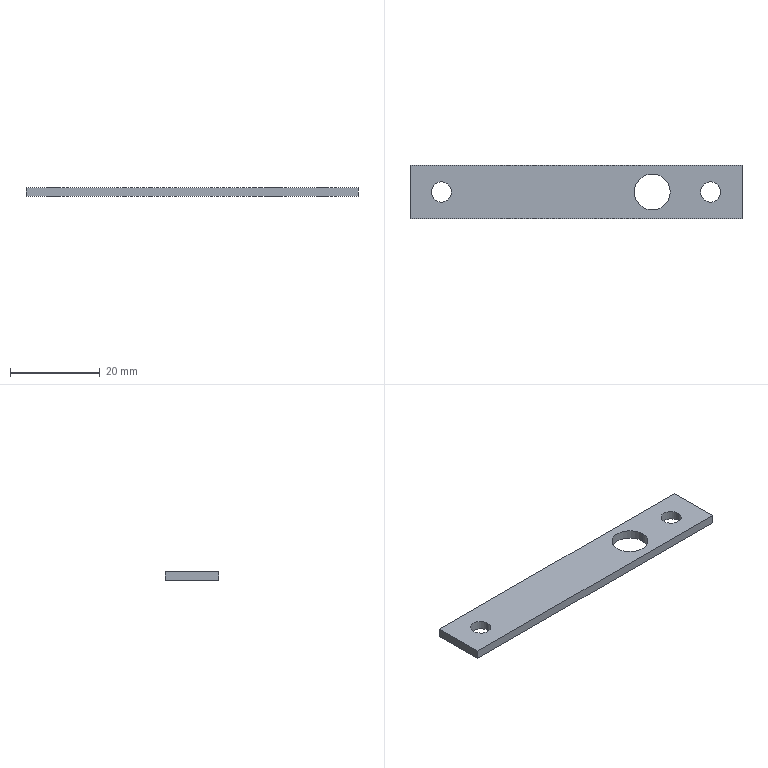Part | Creo | features DATUM PLANE 3, COORDINATE SYSTEM 1, CURVE 1, PROTRUSION 1 | 1 solid | 12 faces | box 74 x 12 x 2 mm | volume 1612 mm3 | plane 6 | cylinder 6 | commonest cylinder face diameters 4.5 x4 8 x2
STEP:
#1=CARTESIAN_POINT('',(0.,0.,0.));
#2=DIRECTION('',(0.,0.,1.));
#3=DIRECTION('',(1.,0.,0.));
#4=AXIS2_PLACEMENT_3D('',#1,#2,#3);
#5=CARTESIAN_POINT('',(-54.,6.,0.));
#6=VERTEX_POINT('',#5);
#7=CARTESIAN_POINT('',(-54.,-6.,0.));
#8=VERTEX_POINT('',#7);
#9=CARTESIAN_POINT('',(-54.,6.,0.));
#10=DIRECTION('',(0.,-1.,0.));
#11=VECTOR('',#10,12.);
#12=LINE('',#9,#11);
#13=EDGE_CURVE('',#6,#8,#12,.T.);
#14=ORIENTED_EDGE('',*,*,#13,.T.);
#15=CARTESIAN_POINT('',(20.,-6.,0.));
#16=VERTEX_POINT('',#15);
#17=CARTESIAN_POINT('',(-54.,-6.,0.));
#18=DIRECTION('',(1.,0.,0.));
#19=VECTOR('',#18,74.);
#20=LINE('',#17,#19);
#21=EDGE_CURVE('',#8,#16,#20,.T.);
#22=ORIENTED_EDGE('',*,*,#21,.T.);
#23=CARTESIAN_POINT('',(20.,6.,0.));
#24=VERTEX_POINT('',#23);
#25=CARTESIAN_POINT('',(20.,-6.,0.));
#26=DIRECTION('',(0.,1.,0.));
#27=VECTOR('',#26,12.);
#28=LINE('',#25,#27);
#29=EDGE_CURVE('',#16,#24,#28,.T.);
#30=ORIENTED_EDGE('',*,*,#29,.T.);
#31=CARTESIAN_POINT('',(20.,6.,0.));
#32=DIRECTION('',(-1.,0.,0.));
#33=VECTOR('',#32,74.);
#34=LINE('',#31,#33);
#35=EDGE_CURVE('',#24,#6,#34,.T.);
#36=ORIENTED_EDGE('',*,*,#35,.T.);
#37=EDGE_LOOP('',(#14,#22,#30,#36));
#38=FACE_OUTER_BOUND('',#37,.F.);
#39=CARTESIAN_POINT('',(15.25,0.,0.));
#40=VERTEX_POINT('',#39);
#41=CARTESIAN_POINT('',(10.75,0.,0.));
#42=VERTEX_POINT('',#41);
#43=CARTESIAN_POINT('',(13.,0.,0.));
#44=DIRECTION('',(0.,0.,-1.));
#45=DIRECTION('',(1.,0.,0.));
#46=AXIS2_PLACEMENT_3D('',#43,#44,#45);
#47=CIRCLE('',#46,2.25);
#48=EDGE_CURVE('',#40,#42,#47,.T.);
#49=ORIENTED_EDGE('',*,*,#48,.T.);
#50=CARTESIAN_POINT('',(13.,0.,0.));
#51=DIRECTION('',(0.,0.,-1.));
#52=DIRECTION('',(-1.,0.,0.));
#53=AXIS2_PLACEMENT_3D('',#50,#51,#52);
#54=CIRCLE('',#53,2.25);
#55=EDGE_CURVE('',#42,#40,#54,.T.);
#56=ORIENTED_EDGE('',*,*,#55,.T.);
#57=EDGE_LOOP('',(#49,#56));
#58=FACE_BOUND('',#57,.F.);
#59=CARTESIAN_POINT('',(-44.75,0.,0.));
#60=VERTEX_POINT('',#59);
#61=CARTESIAN_POINT('',(-49.25,0.,0.));
#62=VERTEX_POINT('',#61);
#63=CARTESIAN_POINT('',(-47.,0.,0.));
#64=DIRECTION('',(0.,0.,-1.));
#65=DIRECTION('',(1.,0.,0.));
#66=AXIS2_PLACEMENT_3D('',#63,#64,#65);
#67=CIRCLE('',#66,2.25);
#68=EDGE_CURVE('',#60,#62,#67,.T.);
#69=ORIENTED_EDGE('',*,*,#68,.T.);
#70=CARTESIAN_POINT('',(-47.,0.,0.));
#71=DIRECTION('',(0.,0.,-1.));
#72=DIRECTION('',(-1.,0.,0.));
#73=AXIS2_PLACEMENT_3D('',#70,#71,#72);
#74=CIRCLE('',#73,2.25);
#75=EDGE_CURVE('',#62,#60,#74,.T.);
#76=ORIENTED_EDGE('',*,*,#75,.T.);
#77=EDGE_LOOP('',(#69,#76));
#78=FACE_BOUND('',#77,.F.);
#79=CARTESIAN_POINT('',(4.,0.,0.));
#80=VERTEX_POINT('',#79);
#81=CARTESIAN_POINT('',(-4.,0.,0.));
#82=VERTEX_POINT('',#81);
#83=CARTESIAN_POINT('',(0.,0.,0.));
#84=DIRECTION('',(0.,0.,-1.));
#85=DIRECTION('',(1.,0.,0.));
#86=AXIS2_PLACEMENT_3D('',#83,#84,#85);
#87=CIRCLE('',#86,4.);
#88=EDGE_CURVE('',#80,#82,#87,.T.);
#89=ORIENTED_EDGE('',*,*,#88,.T.);
#90=CARTESIAN_POINT('',(0.,0.,0.));
#91=DIRECTION('',(0.,0.,-1.));
#92=DIRECTION('',(-1.,0.,0.));
#93=AXIS2_PLACEMENT_3D('',#90,#91,#92);
#94=CIRCLE('',#93,4.);
#95=EDGE_CURVE('',#82,#80,#94,.T.);
#96=ORIENTED_EDGE('',*,*,#95,.T.);
#97=EDGE_LOOP('',(#89,#96));
#98=FACE_BOUND('',#97,.F.);
#99=CARTESIAN_POINT('',(0.,0.,0.));
#100=DIRECTION('',(0.,0.,1.));
#101=DIRECTION('',(1.,0.,0.));
#102=AXIS2_PLACEMENT_3D('',#99,#100,#101);
#103=PLANE('',#102);
#104=ADVANCED_FACE('',(#38,#58,#78,#98),#103,.F.);
#105=ORIENTED_EDGE('',*,*,#88,.F.);
#106=CARTESIAN_POINT('',(4.,0.,2.));
#107=VERTEX_POINT('',#106);
#108=CARTESIAN_POINT('',(4.,0.,0.));
#109=DIRECTION('',(0.,0.,1.));
#110=VECTOR('',#109,2.);
#111=LINE('',#108,#110);
#112=EDGE_CURVE('',#80,#107,#111,.T.);
#113=ORIENTED_EDGE('',*,*,#112,.T.);
#114=CARTESIAN_POINT('',(-4.,0.,2.));
#115=VERTEX_POINT('',#114);
#116=CARTESIAN_POINT('',(0.,0.,2.));
#117=DIRECTION('',(0.,0.,-1.));
#118=DIRECTION('',(1.,0.,0.));
#119=AXIS2_PLACEMENT_3D('',#116,#117,#118);
#120=CIRCLE('',#119,4.);
#121=EDGE_CURVE('',#107,#115,#120,.T.);
#122=ORIENTED_EDGE('',*,*,#121,.T.);
#123=CARTESIAN_POINT('',(-4.,0.,0.));
#124=DIRECTION('',(0.,0.,1.));
#125=VECTOR('',#124,2.);
#126=LINE('',#123,#125);
#127=EDGE_CURVE('',#82,#115,#126,.T.);
#128=ORIENTED_EDGE('',*,*,#127,.F.);
#129=EDGE_LOOP('',(#105,#113,#122,#128));
#130=FACE_OUTER_BOUND('',#129,.F.);
#131=CARTESIAN_POINT('',(0.,0.,0.));
#132=DIRECTION('',(0.,0.,1.));
#133=DIRECTION('',(1.,0.,0.));
#134=AXIS2_PLACEMENT_3D('',#131,#132,#133);
#135=CYLINDRICAL_SURFACE('',#134,4.);
#136=ADVANCED_FACE('',(#130),#135,.F.);
#137=ORIENTED_EDGE('',*,*,#95,.F.);
#138=ORIENTED_EDGE('',*,*,#127,.T.);
#139=CARTESIAN_POINT('',(0.,0.,2.));
#140=DIRECTION('',(0.,0.,-1.));
#141=DIRECTION('',(-1.,0.,0.));
#142=AXIS2_PLACEMENT_3D('',#139,#140,#141);
#143=CIRCLE('',#142,4.);
#144=EDGE_CURVE('',#115,#107,#143,.T.);
#145=ORIENTED_EDGE('',*,*,#144,.T.);
#146=ORIENTED_EDGE('',*,*,#112,.F.);
#147=EDGE_LOOP('',(#137,#138,#145,#146));
#148=FACE_OUTER_BOUND('',#147,.F.);
#149=CARTESIAN_POINT('',(0.,0.,0.));
#150=DIRECTION('',(0.,0.,1.));
#151=DIRECTION('',(1.,0.,0.));
#152=AXIS2_PLACEMENT_3D('',#149,#150,#151);
#153=CYLINDRICAL_SURFACE('',#152,4.);
#154=ADVANCED_FACE('',(#148),#153,.F.);
#155=CARTESIAN_POINT('',(-54.,6.,2.));
#156=VERTEX_POINT('',#155);
#157=CARTESIAN_POINT('',(-54.,-6.,2.));
#158=VERTEX_POINT('',#157);
#159=CARTESIAN_POINT('',(-54.,6.,2.));
#160=DIRECTION('',(0.,-1.,0.));
#161=VECTOR('',#160,12.);
#162=LINE('',#159,#161);
#163=EDGE_CURVE('',#156,#158,#162,.T.);
#164=ORIENTED_EDGE('',*,*,#163,.F.);
#165=CARTESIAN_POINT('',(20.,6.,2.));
#166=VERTEX_POINT('',#165);
#167=CARTESIAN_POINT('',(20.,6.,2.));
#168=DIRECTION('',(-1.,0.,0.));
#169=VECTOR('',#168,74.);
#170=LINE('',#167,#169);
#171=EDGE_CURVE('',#166,#156,#170,.T.);
#172=ORIENTED_EDGE('',*,*,#171,.F.);
#173=CARTESIAN_POINT('',(20.,-6.,2.));
#174=VERTEX_POINT('',#173);
#175=CARTESIAN_POINT('',(20.,-6.,2.));
#176=DIRECTION('',(0.,1.,0.));
#177=VECTOR('',#176,12.);
#178=LINE('',#175,#177);
#179=EDGE_CURVE('',#174,#166,#178,.T.);
#180=ORIENTED_EDGE('',*,*,#179,.F.);
#181=CARTESIAN_POINT('',(-54.,-6.,2.));
#182=DIRECTION('',(1.,0.,0.));
#183=VECTOR('',#182,74.);
#184=LINE('',#181,#183);
#185=EDGE_CURVE('',#158,#174,#184,.T.);
#186=ORIENTED_EDGE('',*,*,#185,.F.);
#187=EDGE_LOOP('',(#164,#172,#180,#186));
#188=FACE_OUTER_BOUND('',#187,.F.);
#189=CARTESIAN_POINT('',(15.25,0.,2.));
#190=VERTEX_POINT('',#189);
#191=CARTESIAN_POINT('',(10.75,0.,2.));
#192=VERTEX_POINT('',#191);
#193=CARTESIAN_POINT('',(13.,0.,2.));
#194=DIRECTION('',(0.,0.,-1.));
#195=DIRECTION('',(1.,0.,0.));
#196=AXIS2_PLACEMENT_3D('',#193,#194,#195);
#197=CIRCLE('',#196,2.25);
#198=EDGE_CURVE('',#190,#192,#197,.T.);
#199=ORIENTED_EDGE('',*,*,#198,.F.);
#200=CARTESIAN_POINT('',(13.,0.,2.));
#201=DIRECTION('',(0.,0.,-1.));
#202=DIRECTION('',(-1.,0.,0.));
#203=AXIS2_PLACEMENT_3D('',#200,#201,#202);
#204=CIRCLE('',#203,2.25);
#205=EDGE_CURVE('',#192,#190,#204,.T.);
#206=ORIENTED_EDGE('',*,*,#205,.F.);
#207=EDGE_LOOP('',(#199,#206));
#208=FACE_BOUND('',#207,.F.);
#209=CARTESIAN_POINT('',(-44.75,0.,2.));
#210=VERTEX_POINT('',#209);
#211=CARTESIAN_POINT('',(-49.25,0.,2.));
#212=VERTEX_POINT('',#211);
#213=CARTESIAN_POINT('',(-47.,0.,2.));
#214=DIRECTION('',(0.,0.,-1.));
#215=DIRECTION('',(1.,0.,0.));
#216=AXIS2_PLACEMENT_3D('',#213,#214,#215);
#217=CIRCLE('',#216,2.25);
#218=EDGE_CURVE('',#210,#212,#217,.T.);
#219=ORIENTED_EDGE('',*,*,#218,.F.);
#220=CARTESIAN_POINT('',(-47.,0.,2.));
#221=DIRECTION('',(0.,0.,-1.));
#222=DIRECTION('',(-1.,0.,0.));
#223=AXIS2_PLACEMENT_3D('',#220,#221,#222);
#224=CIRCLE('',#223,2.25);
#225=EDGE_CURVE('',#212,#210,#224,.T.);
#226=ORIENTED_EDGE('',*,*,#225,.F.);
#227=EDGE_LOOP('',(#219,#226));
#228=FACE_BOUND('',#227,.F.);
#229=ORIENTED_EDGE('',*,*,#121,.F.);
#230=ORIENTED_EDGE('',*,*,#144,.F.);
#231=EDGE_LOOP('',(#229,#230));
#232=FACE_BOUND('',#231,.F.);
#233=CARTESIAN_POINT('',(0.,0.,2.));
#234=DIRECTION('',(0.,0.,1.));
#235=DIRECTION('',(1.,0.,0.));
#236=AXIS2_PLACEMENT_3D('',#233,#234,#235);
#237=PLANE('',#236);
#238=ADVANCED_FACE('',(#188,#208,#228,#232),#237,.T.);
#239=ORIENTED_EDGE('',*,*,#48,.F.);
#240=CARTESIAN_POINT('',(15.25,0.,0.));
#241=DIRECTION('',(0.,0.,1.));
#242=VECTOR('',#241,2.);
#243=LINE('',#240,#242);
#244=EDGE_CURVE('',#40,#190,#243,.T.);
#245=ORIENTED_EDGE('',*,*,#244,.T.);
#246=ORIENTED_EDGE('',*,*,#198,.T.);
#247=CARTESIAN_POINT('',(10.75,0.,0.));
#248=DIRECTION('',(0.,0.,1.));
#249=VECTOR('',#248,2.);
#250=LINE('',#247,#249);
#251=EDGE_CURVE('',#42,#192,#250,.T.);
#252=ORIENTED_EDGE('',*,*,#251,.F.);
#253=EDGE_LOOP('',(#239,#245,#246,#252));
#254=FACE_OUTER_BOUND('',#253,.F.);
#255=CARTESIAN_POINT('',(13.,0.,0.));
#256=DIRECTION('',(0.,0.,1.));
#257=DIRECTION('',(1.,0.,0.));
#258=AXIS2_PLACEMENT_3D('',#255,#256,#257);
#259=CYLINDRICAL_SURFACE('',#258,2.25);
#260=ADVANCED_FACE('',(#254),#259,.F.);
#261=ORIENTED_EDGE('',*,*,#55,.F.);
#262=ORIENTED_EDGE('',*,*,#251,.T.);
#263=ORIENTED_EDGE('',*,*,#205,.T.);
#264=ORIENTED_EDGE('',*,*,#244,.F.);
#265=EDGE_LOOP('',(#261,#262,#263,#264));
#266=FACE_OUTER_BOUND('',#265,.F.);
#267=CARTESIAN_POINT('',(13.,0.,0.));
#268=DIRECTION('',(0.,0.,1.));
#269=DIRECTION('',(1.,0.,0.));
#270=AXIS2_PLACEMENT_3D('',#267,#268,#269);
#271=CYLINDRICAL_SURFACE('',#270,2.25);
#272=ADVANCED_FACE('',(#266),#271,.F.);
#273=ORIENTED_EDGE('',*,*,#68,.F.);
#274=CARTESIAN_POINT('',(-44.75,0.,0.));
#275=DIRECTION('',(0.,0.,1.));
#276=VECTOR('',#275,2.);
#277=LINE('',#274,#276);
#278=EDGE_CURVE('',#60,#210,#277,.T.);
#279=ORIENTED_EDGE('',*,*,#278,.T.);
#280=ORIENTED_EDGE('',*,*,#218,.T.);
#281=CARTESIAN_POINT('',(-49.25,0.,0.));
#282=DIRECTION('',(0.,0.,1.));
#283=VECTOR('',#282,2.);
#284=LINE('',#281,#283);
#285=EDGE_CURVE('',#62,#212,#284,.T.);
#286=ORIENTED_EDGE('',*,*,#285,.F.);
#287=EDGE_LOOP('',(#273,#279,#280,#286));
#288=FACE_OUTER_BOUND('',#287,.F.);
#289=CARTESIAN_POINT('',(-47.,0.,0.));
#290=DIRECTION('',(0.,0.,1.));
#291=DIRECTION('',(1.,0.,0.));
#292=AXIS2_PLACEMENT_3D('',#289,#290,#291);
#293=CYLINDRICAL_SURFACE('',#292,2.25);
#294=ADVANCED_FACE('',(#288),#293,.F.);
#295=ORIENTED_EDGE('',*,*,#75,.F.);
#296=ORIENTED_EDGE('',*,*,#285,.T.);
#297=ORIENTED_EDGE('',*,*,#225,.T.);
#298=ORIENTED_EDGE('',*,*,#278,.F.);
#299=EDGE_LOOP('',(#295,#296,#297,#298));
#300=FACE_OUTER_BOUND('',#299,.F.);
#301=CARTESIAN_POINT('',(-47.,0.,0.));
#302=DIRECTION('',(0.,0.,1.));
#303=DIRECTION('',(1.,0.,0.));
#304=AXIS2_PLACEMENT_3D('',#301,#302,#303);
#305=CYLINDRICAL_SURFACE('',#304,2.25);
#306=ADVANCED_FACE('',(#300),#305,.F.);
#307=ORIENTED_EDGE('',*,*,#13,.F.);
#308=CARTESIAN_POINT('',(-54.,6.,0.));
#309=DIRECTION('',(0.,0.,1.));
#310=VECTOR('',#309,2.);
#311=LINE('',#308,#310);
#312=EDGE_CURVE('',#6,#156,#311,.T.);
#313=ORIENTED_EDGE('',*,*,#312,.T.);
#314=ORIENTED_EDGE('',*,*,#163,.T.);
#315=CARTESIAN_POINT('',(-54.,-6.,0.));
#316=DIRECTION('',(0.,0.,1.));
#317=VECTOR('',#316,2.);
#318=LINE('',#315,#317);
#319=EDGE_CURVE('',#8,#158,#318,.T.);
#320=ORIENTED_EDGE('',*,*,#319,.F.);
#321=EDGE_LOOP('',(#307,#313,#314,#320));
#322=FACE_OUTER_BOUND('',#321,.F.);
#323=CARTESIAN_POINT('',(-54.,6.,0.));
#324=DIRECTION('',(-1.,0.,0.));
#325=DIRECTION('',(0.,-1.,0.));
#326=AXIS2_PLACEMENT_3D('',#323,#324,#325);
#327=PLANE('',#326);
#328=ADVANCED_FACE('',(#322),#327,.T.);
#329=ORIENTED_EDGE('',*,*,#35,.F.);
#330=CARTESIAN_POINT('',(20.,6.,0.));
#331=DIRECTION('',(0.,0.,1.));
#332=VECTOR('',#331,2.);
#333=LINE('',#330,#332);
#334=EDGE_CURVE('',#24,#166,#333,.T.);
#335=ORIENTED_EDGE('',*,*,#334,.T.);
#336=ORIENTED_EDGE('',*,*,#171,.T.);
#337=ORIENTED_EDGE('',*,*,#312,.F.);
#338=EDGE_LOOP('',(#329,#335,#336,#337));
#339=FACE_OUTER_BOUND('',#338,.F.);
#340=CARTESIAN_POINT('',(20.,6.,0.));
#341=DIRECTION('',(0.,1.,0.));
#342=DIRECTION('',(-1.,0.,0.));
#343=AXIS2_PLACEMENT_3D('',#340,#341,#342);
#344=PLANE('',#343);
#345=ADVANCED_FACE('',(#339),#344,.T.);
#346=ORIENTED_EDGE('',*,*,#29,.F.);
#347=CARTESIAN_POINT('',(20.,-6.,0.));
#348=DIRECTION('',(0.,0.,1.));
#349=VECTOR('',#348,2.);
#350=LINE('',#347,#349);
#351=EDGE_CURVE('',#16,#174,#350,.T.);
#352=ORIENTED_EDGE('',*,*,#351,.T.);
#353=ORIENTED_EDGE('',*,*,#179,.T.);
#354=ORIENTED_EDGE('',*,*,#334,.F.);
#355=EDGE_LOOP('',(#346,#352,#353,#354));
#356=FACE_OUTER_BOUND('',#355,.F.);
#357=CARTESIAN_POINT('',(20.,-6.,0.));
#358=DIRECTION('',(1.,0.,0.));
#359=DIRECTION('',(0.,1.,0.));
#360=AXIS2_PLACEMENT_3D('',#357,#358,#359);
#361=PLANE('',#360);
#362=ADVANCED_FACE('',(#356),#361,.T.);
#363=ORIENTED_EDGE('',*,*,#21,.F.);
#364=ORIENTED_EDGE('',*,*,#319,.T.);
#365=ORIENTED_EDGE('',*,*,#185,.T.);
#366=ORIENTED_EDGE('',*,*,#351,.F.);
#367=EDGE_LOOP('',(#363,#364,#365,#366));
#368=FACE_OUTER_BOUND('',#367,.F.);
#369=CARTESIAN_POINT('',(-54.,-6.,0.));
#370=DIRECTION('',(0.,-1.,0.));
#371=DIRECTION('',(1.,0.,0.));
#372=AXIS2_PLACEMENT_3D('',#369,#370,#371);
#373=PLANE('',#372);
#374=ADVANCED_FACE('',(#368),#373,.T.);
#375=CLOSED_SHELL('',(#104,#136,#154,#238,#260,#272,#294,#306,#328,#345,#362,#374));
#376=MANIFOLD_SOLID_BREP('',#375);
#377=(LENGTH_UNIT()NAMED_UNIT(*)SI_UNIT(.MILLI.,.METRE.));
#378=UNCERTAINTY_MEASURE_WITH_UNIT(LENGTH_MEASURE(0.007499),#377,'','');
#379=(NAMED_UNIT(*)PLANE_ANGLE_UNIT()SI_UNIT($,.RADIAN.));
#380=PLANE_ANGLE_MEASURE_WITH_UNIT(PLANE_ANGLE_MEASURE(0.01745),#379);
#381=(CONVERSION_BASED_UNIT('DEGREE',#380)NAMED_UNIT(*)PLANE_ANGLE_UNIT());
#382=(NAMED_UNIT(*)SI_UNIT($,.STERADIAN.)SOLID_ANGLE_UNIT());
#383=(GEOMETRIC_REPRESENTATION_CONTEXT(3)GLOBAL_UNCERTAINTY_ASSIGNED_CONTEXT((#378))GLOBAL_UNIT_ASSIGNED_CONTEXT((#377,#381,#382))REPRESENTATION_CONTEXT('',''));
#384=ADVANCED_BREP_SHAPE_REPRESENTATION('',(#4,#376),#383);